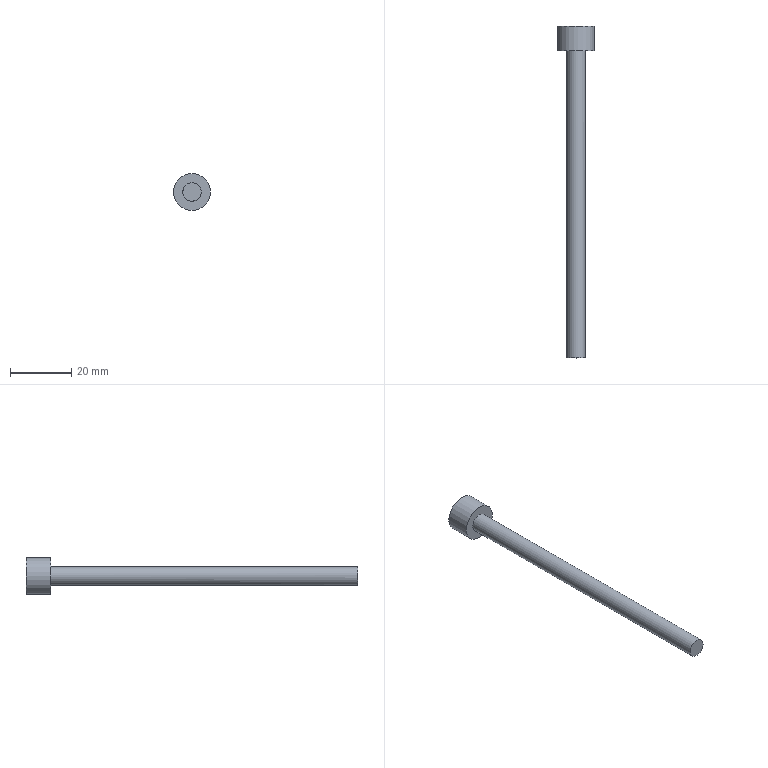Part | STEP file | 1 solid | 5 faces | box 12 x 108 x 12 mm | volume 3732 mm3 | plane 3 | cylinder 2 | commonest cylinder face diameters 6 x1 12 x1
STEP:
#1=CARTESIAN_POINT('',(0.,0.,0.));
#2=DIRECTION('',(0.,0.,1.));
#3=DIRECTION('',(1.,0.,0.));
#4=AXIS2_PLACEMENT_3D('',#1,#2,#3);
#5=CARTESIAN_POINT('',(1700.957,532.48,7.419));
#6=VERTEX_POINT('',#5);
#7=CARTESIAN_POINT('',(1697.957,532.48,10.419));
#8=VERTEX_POINT('',#7);
#9=CARTESIAN_POINT('',(1697.957,532.48,7.419));
#10=DIRECTION('',(0.,1.,0.));
#11=DIRECTION('',(1.,0.,0.));
#12=AXIS2_PLACEMENT_3D('',#9,#10,#11);
#13=CIRCLE('',#12,3.);
#14=CARTESIAN_POINT('',(1697.957,532.48,7.419));
#15=DIRECTION('',(0.,-1.,0.));
#16=DIRECTION('',(0.,0.,-1.));
#17=AXIS2_PLACEMENT_3D('',#14,#15,#16);
#18=PLANE('',#17);
#19=CARTESIAN_POINT('',(0.,3.));
#20=CARTESIAN_POINT('',(5.196,3.));
#21=CARTESIAN_POINT('',(2.598,-1.5));
#22=CARTESIAN_POINT('',(0.,-6.));
#23=CARTESIAN_POINT('',(-2.598,-1.5));
#24=CARTESIAN_POINT('',(-5.196,3.));
#25=CARTESIAN_POINT('',(0.,3.));
#26=(BOUNDED_CURVE()B_SPLINE_CURVE(2,(#19,#20,#21,#22,#23,#24,#25),.UNSPECIFIED.,.T.,.F.)B_SPLINE_CURVE_WITH_KNOTS((1,2,2,2,2,1),(-2.094,0.,2.094,4.189,6.283,8.378),.UNSPECIFIED.)CURVE()GEOMETRIC_REPRESENTATION_ITEM()RATIONAL_B_SPLINE_CURVE((1.,0.5,1.,0.5,1.,0.5,1.))REPRESENTATION_ITEM(''));
#27=(GEOMETRIC_REPRESENTATION_CONTEXT(2)PARAMETRIC_REPRESENTATION_CONTEXT()REPRESENTATION_CONTEXT('',''));
#28=DEFINITIONAL_REPRESENTATION('',(#26),#27);
#29=PCURVE('',#18,#28);
#30=CARTESIAN_POINT('',(1697.957,582.48,7.419));
#31=DIRECTION('',(0.,-1.,0.));
#32=DIRECTION('',(-1.,0.,0.));
#33=AXIS2_PLACEMENT_3D('',#30,#31,#32);
#34=CYLINDRICAL_SURFACE('',#33,3.);
#35=CARTESIAN_POINT('',(9.425,50.));
#36=DIRECTION('',(-1.,0.));
#37=VECTOR('',#36,1.);
#38=LINE('',#35,#37);
#39=(GEOMETRIC_REPRESENTATION_CONTEXT(2)PARAMETRIC_REPRESENTATION_CONTEXT()REPRESENTATION_CONTEXT('',''));
#40=DEFINITIONAL_REPRESENTATION('',(#38),#39);
#41=PCURVE('',#34,#40);
#42=SURFACE_CURVE('',#13,(#29,#41),.PCURVE_S1.);
#43=EDGE_CURVE('',#6,#8,#42,.T.);
#44=ORIENTED_EDGE('',*,*,#43,.F.);
#45=CARTESIAN_POINT('',(1697.957,532.48,7.419));
#46=DIRECTION('',(0.,1.,0.));
#47=DIRECTION('',(1.,0.,0.));
#48=AXIS2_PLACEMENT_3D('',#45,#46,#47);
#49=CIRCLE('',#48,3.);
#50=CARTESIAN_POINT('',(0.,3.));
#51=CARTESIAN_POINT('',(5.196,3.));
#52=CARTESIAN_POINT('',(2.598,-1.5));
#53=CARTESIAN_POINT('',(0.,-6.));
#54=CARTESIAN_POINT('',(-2.598,-1.5));
#55=CARTESIAN_POINT('',(-5.196,3.));
#56=CARTESIAN_POINT('',(0.,3.));
#57=(BOUNDED_CURVE()B_SPLINE_CURVE(2,(#50,#51,#52,#53,#54,#55,#56),.UNSPECIFIED.,.T.,.F.)B_SPLINE_CURVE_WITH_KNOTS((1,2,2,2,2,1),(-2.094,0.,2.094,4.189,6.283,8.378),.UNSPECIFIED.)CURVE()GEOMETRIC_REPRESENTATION_ITEM()RATIONAL_B_SPLINE_CURVE((1.,0.5,1.,0.5,1.,0.5,1.))REPRESENTATION_ITEM(''));
#58=(GEOMETRIC_REPRESENTATION_CONTEXT(2)PARAMETRIC_REPRESENTATION_CONTEXT()REPRESENTATION_CONTEXT('',''));
#59=DEFINITIONAL_REPRESENTATION('',(#57),#58);
#60=PCURVE('',#18,#59);
#61=CARTESIAN_POINT('',(15.708,50.));
#62=DIRECTION('',(-1.,0.));
#63=VECTOR('',#62,1.);
#64=LINE('',#61,#63);
#65=(GEOMETRIC_REPRESENTATION_CONTEXT(2)PARAMETRIC_REPRESENTATION_CONTEXT()REPRESENTATION_CONTEXT('',''));
#66=DEFINITIONAL_REPRESENTATION('',(#64),#65);
#67=PCURVE('',#34,#66);
#68=SURFACE_CURVE('',#49,(#60,#67),.PCURVE_S1.);
#69=EDGE_CURVE('',#8,#6,#68,.T.);
#70=ORIENTED_EDGE('',*,*,#69,.F.);
#71=EDGE_LOOP('',(#44,#70));
#72=FACE_BOUND('',#71,.T.);
#73=ADVANCED_FACE('',(#72),#18,.T.);
#74=ORIENTED_EDGE('',*,*,#43,.T.);
#75=CARTESIAN_POINT('',(1697.957,632.48,10.419));
#76=VERTEX_POINT('',#75);
#77=CARTESIAN_POINT('',(1697.957,632.48,10.419));
#78=CARTESIAN_POINT('',(1697.957,532.48,10.419));
#79=B_SPLINE_CURVE_WITH_KNOTS('',1,(#77,#78),.UNSPECIFIED.,.F.,.F.,(2,2),(-50.,50.),.PIECEWISE_BEZIER_KNOTS.);
#80=CARTESIAN_POINT('',(4.712,0.));
#81=DIRECTION('',(0.,1.));
#82=VECTOR('',#81,1.);
#83=LINE('',#80,#82);
#84=(GEOMETRIC_REPRESENTATION_CONTEXT(2)PARAMETRIC_REPRESENTATION_CONTEXT()REPRESENTATION_CONTEXT('',''));
#85=DEFINITIONAL_REPRESENTATION('',(#83),#84);
#86=PCURVE('',#34,#85);
#87=CARTESIAN_POINT('',(10.996,0.));
#88=DIRECTION('',(0.,1.));
#89=VECTOR('',#88,1.);
#90=LINE('',#87,#89);
#91=(GEOMETRIC_REPRESENTATION_CONTEXT(2)PARAMETRIC_REPRESENTATION_CONTEXT()REPRESENTATION_CONTEXT('',''));
#92=DEFINITIONAL_REPRESENTATION('',(#90),#91);
#93=PCURVE('',#34,#92);
#94=SEAM_CURVE('',#79,(#86,#93),.PCURVE_S1.);
#95=EDGE_CURVE('',#76,#8,#94,.T.);
#96=ORIENTED_EDGE('',*,*,#95,.F.);
#97=CARTESIAN_POINT('',(1697.957,632.48,7.419));
#98=DIRECTION('',(0.,1.,0.));
#99=DIRECTION('',(0.,0.,1.));
#100=AXIS2_PLACEMENT_3D('',#97,#98,#99);
#101=CIRCLE('',#100,3.);
#102=CARTESIAN_POINT('',(10.996,-50.));
#103=DIRECTION('',(-1.,0.));
#104=VECTOR('',#103,1.);
#105=LINE('',#102,#104);
#106=(GEOMETRIC_REPRESENTATION_CONTEXT(2)PARAMETRIC_REPRESENTATION_CONTEXT()REPRESENTATION_CONTEXT('',''));
#107=DEFINITIONAL_REPRESENTATION('',(#105),#106);
#108=PCURVE('',#34,#107);
#109=CARTESIAN_POINT('',(1697.957,632.48,7.419));
#110=DIRECTION('',(0.,-1.,0.));
#111=DIRECTION('',(0.,0.,-1.));
#112=AXIS2_PLACEMENT_3D('',#109,#110,#111);
#113=PLANE('',#112);
#114=CARTESIAN_POINT('',(-3.,0.));
#115=CARTESIAN_POINT('',(-3.,5.196));
#116=CARTESIAN_POINT('',(1.5,2.598));
#117=CARTESIAN_POINT('',(6.,0.));
#118=CARTESIAN_POINT('',(1.5,-2.598));
#119=CARTESIAN_POINT('',(-3.,-5.196));
#120=CARTESIAN_POINT('',(-3.,0.));
#121=(BOUNDED_CURVE()B_SPLINE_CURVE(2,(#114,#115,#116,#117,#118,#119,#120),.UNSPECIFIED.,.T.,.F.)B_SPLINE_CURVE_WITH_KNOTS((1,2,2,2,2,1),(-2.094,0.,2.094,4.189,6.283,8.378),.UNSPECIFIED.)CURVE()GEOMETRIC_REPRESENTATION_ITEM()RATIONAL_B_SPLINE_CURVE((1.,0.5,1.,0.5,1.,0.5,1.))REPRESENTATION_ITEM(''));
#122=(GEOMETRIC_REPRESENTATION_CONTEXT(2)PARAMETRIC_REPRESENTATION_CONTEXT()REPRESENTATION_CONTEXT('',''));
#123=DEFINITIONAL_REPRESENTATION('',(#121),#122);
#124=PCURVE('',#113,#123);
#125=SURFACE_CURVE('',#101,(#108,#124),.PCURVE_S1.);
#126=EDGE_CURVE('',#76,#76,#125,.T.);
#127=ORIENTED_EDGE('',*,*,#126,.F.);
#128=ORIENTED_EDGE('',*,*,#95,.T.);
#129=ORIENTED_EDGE('',*,*,#69,.T.);
#130=EDGE_LOOP('',(#74,#96,#127,#128,#129));
#131=FACE_BOUND('',#130,.T.);
#132=ADVANCED_FACE('',(#131),#34,.T.);
#133=CARTESIAN_POINT('',(1703.957,640.48,7.419));
#134=VERTEX_POINT('',#133);
#135=CARTESIAN_POINT('',(1697.957,640.48,7.419));
#136=DIRECTION('',(0.,-1.,0.));
#137=DIRECTION('',(1.,0.,0.));
#138=AXIS2_PLACEMENT_3D('',#135,#136,#137);
#139=CIRCLE('',#138,6.);
#140=CARTESIAN_POINT('',(1697.957,640.48,7.419));
#141=DIRECTION('',(0.,1.,0.));
#142=DIRECTION('',(0.,0.,1.));
#143=AXIS2_PLACEMENT_3D('',#140,#141,#142);
#144=PLANE('',#143);
#145=CARTESIAN_POINT('',(0.,6.));
#146=CARTESIAN_POINT('',(10.392,6.));
#147=CARTESIAN_POINT('',(5.196,-3.));
#148=CARTESIAN_POINT('',(0.,-12.));
#149=CARTESIAN_POINT('',(-5.196,-3.));
#150=CARTESIAN_POINT('',(-10.392,6.));
#151=CARTESIAN_POINT('',(0.,6.));
#152=(BOUNDED_CURVE()B_SPLINE_CURVE(2,(#145,#146,#147,#148,#149,#150,#151),.UNSPECIFIED.,.T.,.F.)B_SPLINE_CURVE_WITH_KNOTS((1,2,2,2,2,1),(-2.094,0.,2.094,4.189,6.283,8.378),.UNSPECIFIED.)CURVE()GEOMETRIC_REPRESENTATION_ITEM()RATIONAL_B_SPLINE_CURVE((1.,0.5,1.,0.5,1.,0.5,1.))REPRESENTATION_ITEM(''));
#153=(GEOMETRIC_REPRESENTATION_CONTEXT(2)PARAMETRIC_REPRESENTATION_CONTEXT()REPRESENTATION_CONTEXT('',''));
#154=DEFINITIONAL_REPRESENTATION('',(#152),#153);
#155=PCURVE('',#144,#154);
#156=CARTESIAN_POINT('',(1697.957,632.48,7.419));
#157=DIRECTION('',(0.,1.,0.));
#158=DIRECTION('',(-1.,0.,0.));
#159=AXIS2_PLACEMENT_3D('',#156,#157,#158);
#160=CYLINDRICAL_SURFACE('',#159,6.);
#161=CARTESIAN_POINT('',(9.425,8.));
#162=DIRECTION('',(-1.,0.));
#163=VECTOR('',#162,1.);
#164=LINE('',#161,#163);
#165=(GEOMETRIC_REPRESENTATION_CONTEXT(2)PARAMETRIC_REPRESENTATION_CONTEXT()REPRESENTATION_CONTEXT('',''));
#166=DEFINITIONAL_REPRESENTATION('',(#164),#165);
#167=PCURVE('',#160,#166);
#168=SURFACE_CURVE('',#139,(#155,#167),.PCURVE_S1.);
#169=EDGE_CURVE('',#134,#134,#168,.T.);
#170=ORIENTED_EDGE('',*,*,#169,.F.);
#171=EDGE_LOOP('',(#170));
#172=FACE_BOUND('',#171,.T.);
#173=ADVANCED_FACE('',(#172),#144,.T.);
#174=ORIENTED_EDGE('',*,*,#126,.T.);
#175=EDGE_LOOP('',(#174));
#176=FACE_BOUND('',#175,.T.);
#177=CARTESIAN_POINT('',(1703.957,632.48,7.419));
#178=VERTEX_POINT('',#177);
#179=CARTESIAN_POINT('',(1697.957,632.48,7.419));
#180=DIRECTION('',(0.,1.,0.));
#181=DIRECTION('',(1.,0.,0.));
#182=AXIS2_PLACEMENT_3D('',#179,#180,#181);
#183=CIRCLE('',#182,6.);
#184=CARTESIAN_POINT('',(0.,6.));
#185=CARTESIAN_POINT('',(10.392,6.));
#186=CARTESIAN_POINT('',(5.196,-3.));
#187=CARTESIAN_POINT('',(0.,-12.));
#188=CARTESIAN_POINT('',(-5.196,-3.));
#189=CARTESIAN_POINT('',(-10.392,6.));
#190=CARTESIAN_POINT('',(0.,6.));
#191=(BOUNDED_CURVE()B_SPLINE_CURVE(2,(#184,#185,#186,#187,#188,#189,#190),.UNSPECIFIED.,.T.,.F.)B_SPLINE_CURVE_WITH_KNOTS((1,2,2,2,2,1),(-2.094,0.,2.094,4.189,6.283,8.378),.UNSPECIFIED.)CURVE()GEOMETRIC_REPRESENTATION_ITEM()RATIONAL_B_SPLINE_CURVE((1.,0.5,1.,0.5,1.,0.5,1.))REPRESENTATION_ITEM(''));
#192=(GEOMETRIC_REPRESENTATION_CONTEXT(2)PARAMETRIC_REPRESENTATION_CONTEXT()REPRESENTATION_CONTEXT('',''));
#193=DEFINITIONAL_REPRESENTATION('',(#191),#192);
#194=PCURVE('',#113,#193);
#195=CARTESIAN_POINT('',(3.142,0.));
#196=DIRECTION('',(1.,0.));
#197=VECTOR('',#196,1.);
#198=LINE('',#195,#197);
#199=(GEOMETRIC_REPRESENTATION_CONTEXT(2)PARAMETRIC_REPRESENTATION_CONTEXT()REPRESENTATION_CONTEXT('',''));
#200=DEFINITIONAL_REPRESENTATION('',(#198),#199);
#201=PCURVE('',#160,#200);
#202=SURFACE_CURVE('',#183,(#194,#201),.PCURVE_S1.);
#203=EDGE_CURVE('',#178,#178,#202,.T.);
#204=ORIENTED_EDGE('',*,*,#203,.F.);
#205=EDGE_LOOP('',(#204));
#206=FACE_BOUND('',#205,.T.);
#207=ADVANCED_FACE('',(#176,#206),#113,.T.);
#208=ORIENTED_EDGE('',*,*,#169,.T.);
#209=CARTESIAN_POINT('',(1703.957,632.48,7.419));
#210=CARTESIAN_POINT('',(1703.957,640.48,7.419));
#211=B_SPLINE_CURVE_WITH_KNOTS('',1,(#209,#210),.UNSPECIFIED.,.F.,.F.,(2,2),(0.,8.),.PIECEWISE_BEZIER_KNOTS.);
#212=CARTESIAN_POINT('',(3.142,0.));
#213=DIRECTION('',(0.,1.));
#214=VECTOR('',#213,1.);
#215=LINE('',#212,#214);
#216=(GEOMETRIC_REPRESENTATION_CONTEXT(2)PARAMETRIC_REPRESENTATION_CONTEXT()REPRESENTATION_CONTEXT('',''));
#217=DEFINITIONAL_REPRESENTATION('',(#215),#216);
#218=PCURVE('',#160,#217);
#219=CARTESIAN_POINT('',(9.425,0.));
#220=DIRECTION('',(0.,1.));
#221=VECTOR('',#220,1.);
#222=LINE('',#219,#221);
#223=(GEOMETRIC_REPRESENTATION_CONTEXT(2)PARAMETRIC_REPRESENTATION_CONTEXT()REPRESENTATION_CONTEXT('',''));
#224=DEFINITIONAL_REPRESENTATION('',(#222),#223);
#225=PCURVE('',#160,#224);
#226=SEAM_CURVE('',#211,(#218,#225),.PCURVE_S1.);
#227=EDGE_CURVE('',#178,#134,#226,.T.);
#228=ORIENTED_EDGE('',*,*,#227,.F.);
#229=ORIENTED_EDGE('',*,*,#203,.T.);
#230=ORIENTED_EDGE('',*,*,#227,.T.);
#231=EDGE_LOOP('',(#208,#228,#229,#230));
#232=FACE_BOUND('',#231,.T.);
#233=ADVANCED_FACE('',(#232),#160,.T.);
#234=CLOSED_SHELL('',(#73,#132,#173,#207,#233));
#235=MANIFOLD_SOLID_BREP('',#234);
#236=(LENGTH_UNIT()NAMED_UNIT(*)SI_UNIT(.MILLI.,.METRE.));
#237=UNCERTAINTY_MEASURE_WITH_UNIT(LENGTH_MEASURE(0.000005),#236,'','');
#238=(NAMED_UNIT(*)PLANE_ANGLE_UNIT()SI_UNIT($,.RADIAN.));
#239=(NAMED_UNIT(*)SI_UNIT($,.STERADIAN.)SOLID_ANGLE_UNIT());
#240=(GEOMETRIC_REPRESENTATION_CONTEXT(3)GLOBAL_UNCERTAINTY_ASSIGNED_CONTEXT((#237))GLOBAL_UNIT_ASSIGNED_CONTEXT((#236,#238,#239))REPRESENTATION_CONTEXT('',''));
#241=ADVANCED_BREP_SHAPE_REPRESENTATION('',(#4,#235),#240);